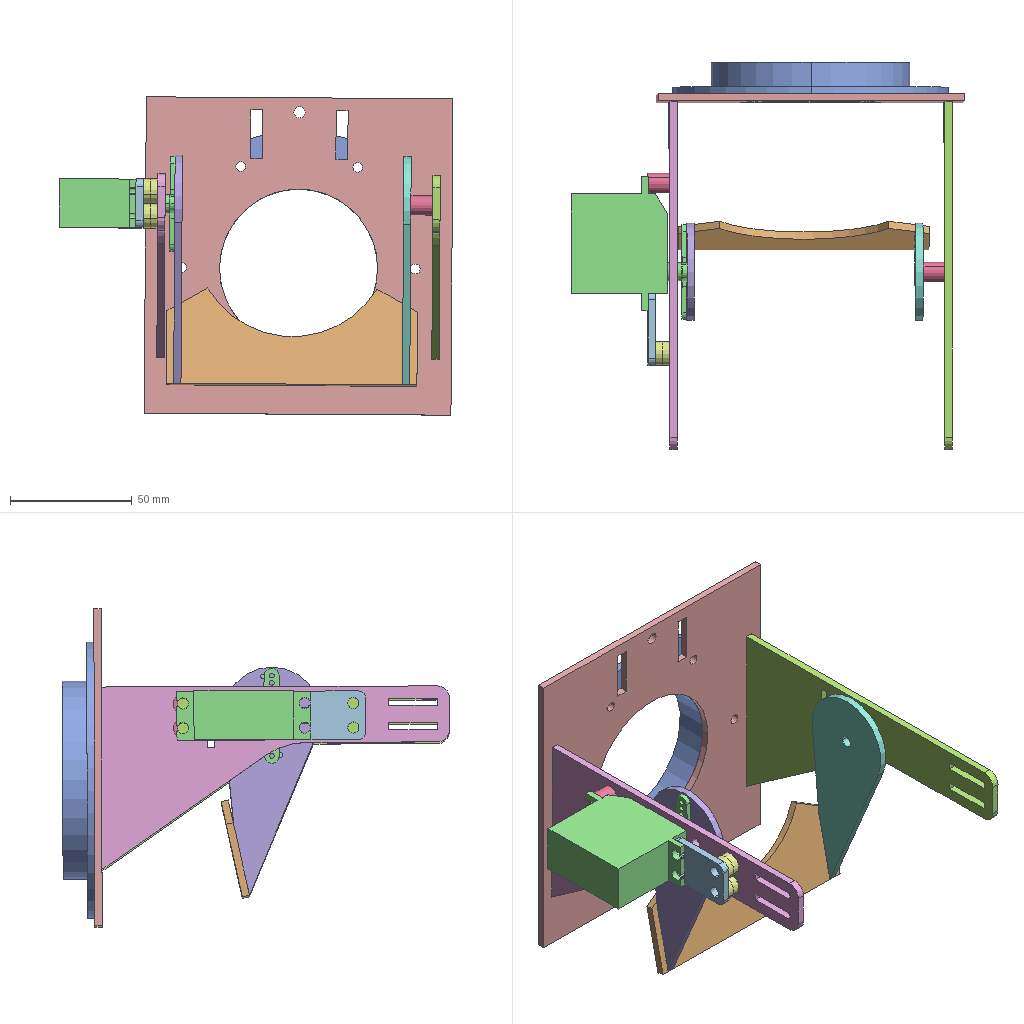Assembly | SolidWorks | 11 different items | 16 placed | box 162 x 159 x 131 mm
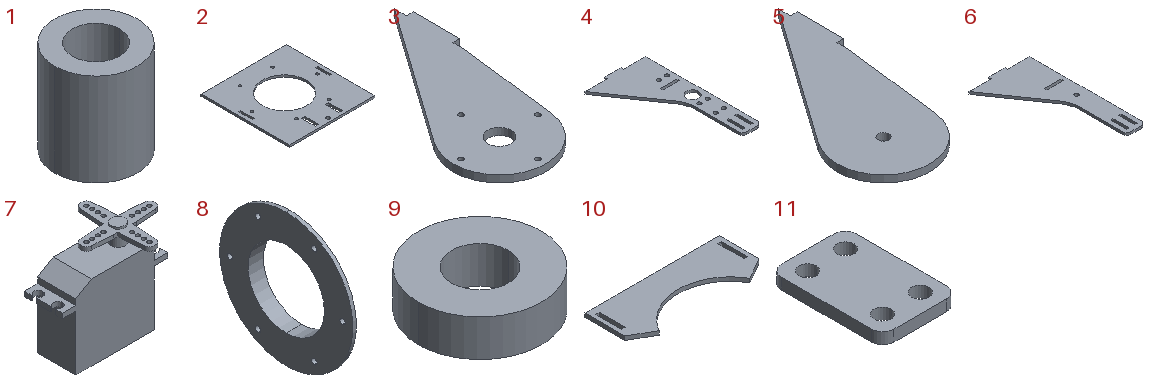Parts list (item | quantity | size | volume | features):
1 | x3 | 8 x 8 x 9 mm | 302.818 mm3 | features Extrusion 1
2 | x1 | 126 x 130 x 3 mm | 37973 mm3 | features Cut 2, Extrusion 1, HoleWzd 1, MirrorPattern 1
3 | x1 | 48 x 90 x 3 mm | 6643 mm3 | features ICE 3, Extrusion 1
4 | x1 | 75 x 146 x 3 mm | 14540 mm3 | features Cut 3, Fillet 2, Extrusion 1
5 | x1 | 48 x 90 x 3 mm | 6866 mm3 | features ICE 2, Extrusion 1
6 | x1 | 75 x 146 x 3 mm | 15319 mm3 | features Fillet 2, Cut 1, Extrusion 1, ICE 1
7 | x1 | 58.5 x 39 x 48.5 mm | 33649 mm3 | features ICE 6, Fillet 2, Chamfer 1, Extrusion 1, MirrorPattern 1
8 | x1 | 13 x 113.5 x 113.5 mm | 34508 mm3 | features Chamfer 2, CirPattern 1, ICE 1, Revolution 1
9 | x4 | 10 x 10 x 3 mm | 185.762 mm3 | features Extrusion 1
10 | x1 | 102.9 x 40.212 x 3 mm | 8591 mm3 | features Extrusion 1, ICE 1
11 | x1 | 20 x 30 x 3 mm | 1577 mm3 | features Extrusion 1, Fillet 1, ICE 1
Mates (type | each side: item.copy, entity, surface, feature):
Coincident | 2.1 face plane Boss-Extrude1 | 8.1 face plane Revolve1
Concentric | 2.1 face cylinder Boss-Extrude1 | 8.1 face cylinder Revolve1
Concentric | 2.1 face cylinder Ø4.0 (4) Diameter Hole1 | 8.1 face cylinder Cut-Extrude1
Parallel | 2.1 face plane Boss-Extrude1 | 6.1 face plane Boss-Extrude1
Coincident | 2.1 face plane Boss-Extrude1 | 6.1 face plane Boss-Extrude1
DistanceDim | 2.1 face plane Cut-Extrude1 | 4.1 face plane Boss-Extrude1
Coincident | 2.1 face plane Cut-Extrude1 | 4.1 face plane Boss-Extrude1
Coincident | 5.1 face plane Boss-Extrude1 | 10.1 face plane Boss-Extrude1
Coincident | 5.1 face plane Boss-Extrude3 | 10.1 face plane Boss-Extrude1
DistanceDim | 5.1 face plane Boss-Extrude1 | 10.1 face plane Boss-Extrude1
Coincident | 10.1 face plane Boss-Extrude1 | 3.1 face plane Boss-Extrude1
Coincident | 10.1 face plane Boss-Extrude1 | 3.1 face plane Boss-Extrude3
DistanceDim | 10.1 face plane Boss-Extrude1 | 3.1 face plane Boss-Extrude1
DistanceDim | 4.1 face plane Boss-Extrude1 | 7.1 face plane Boss-Extrude2
Concentric | 4.1 edge | 7.1 face cylinder Boss-Extrude3
Concentric | 7.1 face cylinder Boss-Extrude5 | 3.1 face cylinder Cut-Extrude1
Coincident | 7.1 face plane Boss-Extrude3 | 3.1 face plane Boss-Extrude1
Concentric | 4.1 face cylinder Cut-Extrude1 | 1.1 face cylinder Boss-Extrude1
Concentric | 7.1 face cylinder Cut-Extrude1 | 1.1 face cylinder Boss-Extrude1
Coincident | 7.1 face plane Boss-Extrude2 | 1.1 face plane Boss-Extrude1
Concentric | 7.1 face cylinder Cut-Extrude1 | 1.2 face cylinder Boss-Extrude1
Coincident | 7.1 face plane Boss-Extrude2 | 1.2 face plane Boss-Extrude1
Concentric | 6.1 face cylinder Cut-Extrude1 | 1.3 face cylinder Boss-Extrude1
Coincident | 6.1 face plane Boss-Extrude1 | 1.3 face plane Boss-Extrude1
Concentric | 5.1 face cylinder Cut-Extrude1 | 1.3 face cylinder Boss-Extrude1
Coincident | 5.1 face plane Boss-Extrude1 | 1.3 face plane Boss-Extrude1
Coincident | 7.1 face plane Boss-Extrude2 | 11.1 face plane Boss-Extrude1
Concentric | 7.1 face cylinder Mirror1 | 11.1 face cylinder Cut-Extrude1 | 2 times
Concentric | 11.1 face cylinder Cut-Extrude1 | 9.1 face cylinder Boss-Extrude1
Coincident | 11.1 face plane Boss-Extrude1 | 9.1 face plane Boss-Extrude1